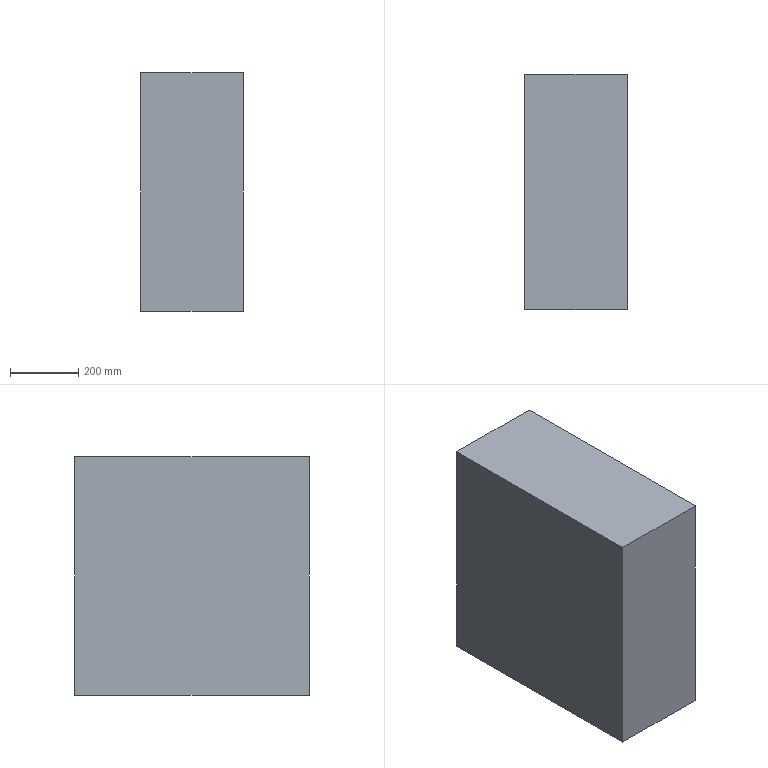Part | SolidWorks | features ICE 2, Extrusion 1 | 1 solid | 16 faces | box 300 x 690 x 700 mm | volume 37296000 mm3 | plane 16
STEP:
#1=CARTESIAN_POINT('',(-150.,345.,0.));
#2=VERTEX_POINT('',#1);
#3=CARTESIAN_POINT('',(-150.,-345.,0.));
#4=VERTEX_POINT('',#3);
#5=CARTESIAN_POINT('',(-150.,-345.,0.));
#6=DIRECTION('',(0.,-1.,0.));
#7=VECTOR('',#6,1000.);
#8=LINE('',#5,#7);
#9=EDGE_CURVE('',#2,#4,#8,.T.);
#10=ORIENTED_EDGE('',*,*,#9,.T.);
#11=CARTESIAN_POINT('',(-150.,-345.,700.));
#12=VERTEX_POINT('',#11);
#13=CARTESIAN_POINT('',(-150.,-345.,700.));
#14=DIRECTION('',(0.,0.,-1.));
#15=VECTOR('',#14,1000.);
#16=LINE('',#13,#15);
#17=EDGE_CURVE('',#12,#4,#16,.T.);
#18=ORIENTED_EDGE('',*,*,#17,.F.);
#19=CARTESIAN_POINT('',(-150.,345.,700.));
#20=VERTEX_POINT('',#19);
#21=CARTESIAN_POINT('',(-150.,-345.,700.));
#22=DIRECTION('',(0.,-1.,0.));
#23=VECTOR('',#22,1000.);
#24=LINE('',#21,#23);
#25=EDGE_CURVE('',#20,#12,#24,.T.);
#26=ORIENTED_EDGE('',*,*,#25,.F.);
#27=CARTESIAN_POINT('',(-150.,345.,700.));
#28=DIRECTION('',(0.,0.,-1.));
#29=VECTOR('',#28,1000.);
#30=LINE('',#27,#29);
#31=EDGE_CURVE('',#20,#2,#30,.T.);
#32=ORIENTED_EDGE('',*,*,#31,.T.);
#33=EDGE_LOOP('',(#10,#18,#26,#32));
#34=FACE_OUTER_BOUND('',#33,.T.);
#35=CARTESIAN_POINT('',(-150.,-345.,700.));
#36=DIRECTION('',(1.,0.,0.));
#37=DIRECTION('',(0.,0.,-1.));
#38=AXIS2_PLACEMENT_3D('',#35,#36,#37);
#39=PLANE('',#38);
#40=ADVANCED_FACE('',(#34),#39,.F.);
#41=CARTESIAN_POINT('',(150.,-345.,0.));
#42=VERTEX_POINT('',#41);
#43=CARTESIAN_POINT('',(150.,-345.,0.));
#44=DIRECTION('',(1.,0.,0.));
#45=VECTOR('',#44,1000.);
#46=LINE('',#43,#45);
#47=EDGE_CURVE('',#4,#42,#46,.T.);
#48=ORIENTED_EDGE('',*,*,#47,.T.);
#49=CARTESIAN_POINT('',(150.,-345.,700.));
#50=VERTEX_POINT('',#49);
#51=CARTESIAN_POINT('',(150.,-345.,700.));
#52=DIRECTION('',(0.,0.,-1.));
#53=VECTOR('',#52,1000.);
#54=LINE('',#51,#53);
#55=EDGE_CURVE('',#50,#42,#54,.T.);
#56=ORIENTED_EDGE('',*,*,#55,.F.);
#57=CARTESIAN_POINT('',(150.,-345.,700.));
#58=DIRECTION('',(1.,0.,0.));
#59=VECTOR('',#58,1000.);
#60=LINE('',#57,#59);
#61=EDGE_CURVE('',#12,#50,#60,.T.);
#62=ORIENTED_EDGE('',*,*,#61,.F.);
#63=ORIENTED_EDGE('',*,*,#17,.T.);
#64=EDGE_LOOP('',(#48,#56,#62,#63));
#65=FACE_OUTER_BOUND('',#64,.T.);
#66=CARTESIAN_POINT('',(150.,-345.,700.));
#67=DIRECTION('',(0.,1.,0.));
#68=DIRECTION('',(0.,0.,1.));
#69=AXIS2_PLACEMENT_3D('',#66,#67,#68);
#70=PLANE('',#69);
#71=ADVANCED_FACE('',(#65),#70,.F.);
#72=CARTESIAN_POINT('',(150.,-325.,665.));
#73=VERTEX_POINT('',#72);
#74=CARTESIAN_POINT('',(150.,-325.,35.));
#75=VERTEX_POINT('',#74);
#76=CARTESIAN_POINT('',(150.,-325.,35.));
#77=DIRECTION('',(0.,0.,-1.));
#78=VECTOR('',#77,1000.);
#79=LINE('',#76,#78);
#80=EDGE_CURVE('',#73,#75,#79,.T.);
#81=ORIENTED_EDGE('',*,*,#80,.F.);
#82=CARTESIAN_POINT('',(150.,135.,665.));
#83=VERTEX_POINT('',#82);
#84=CARTESIAN_POINT('',(150.,-325.,665.));
#85=DIRECTION('',(0.,-1.,0.));
#86=VECTOR('',#85,1000.);
#87=LINE('',#84,#86);
#88=EDGE_CURVE('',#83,#73,#87,.T.);
#89=ORIENTED_EDGE('',*,*,#88,.F.);
#90=CARTESIAN_POINT('',(150.,135.,35.));
#91=VERTEX_POINT('',#90);
#92=CARTESIAN_POINT('',(150.,135.,35.));
#93=DIRECTION('',(0.,0.,1.));
#94=VECTOR('',#93,1000.);
#95=LINE('',#92,#94);
#96=EDGE_CURVE('',#91,#83,#95,.T.);
#97=ORIENTED_EDGE('',*,*,#96,.F.);
#98=CARTESIAN_POINT('',(150.,-325.,35.));
#99=DIRECTION('',(0.,1.,0.));
#100=VECTOR('',#99,1000.);
#101=LINE('',#98,#100);
#102=EDGE_CURVE('',#75,#91,#101,.T.);
#103=ORIENTED_EDGE('',*,*,#102,.F.);
#104=EDGE_LOOP('',(#81,#89,#97,#103));
#105=FACE_BOUND('',#104,.T.);
#106=CARTESIAN_POINT('',(150.,175.,665.));
#107=VERTEX_POINT('',#106);
#108=CARTESIAN_POINT('',(150.,175.,35.));
#109=VERTEX_POINT('',#108);
#110=CARTESIAN_POINT('',(150.,175.,35.));
#111=DIRECTION('',(0.,0.,-1.));
#112=VECTOR('',#111,1000.);
#113=LINE('',#110,#112);
#114=EDGE_CURVE('',#107,#109,#113,.T.);
#115=ORIENTED_EDGE('',*,*,#114,.F.);
#116=CARTESIAN_POINT('',(150.,325.,665.));
#117=VERTEX_POINT('',#116);
#118=CARTESIAN_POINT('',(150.,175.,665.));
#119=DIRECTION('',(0.,-1.,0.));
#120=VECTOR('',#119,1000.);
#121=LINE('',#118,#120);
#122=EDGE_CURVE('',#117,#107,#121,.T.);
#123=ORIENTED_EDGE('',*,*,#122,.F.);
#124=CARTESIAN_POINT('',(150.,325.,35.));
#125=VERTEX_POINT('',#124);
#126=CARTESIAN_POINT('',(150.,325.,35.));
#127=DIRECTION('',(0.,0.,1.));
#128=VECTOR('',#127,1000.);
#129=LINE('',#126,#128);
#130=EDGE_CURVE('',#125,#117,#129,.T.);
#131=ORIENTED_EDGE('',*,*,#130,.F.);
#132=CARTESIAN_POINT('',(150.,175.,35.));
#133=DIRECTION('',(0.,1.,0.));
#134=VECTOR('',#133,1000.);
#135=LINE('',#132,#134);
#136=EDGE_CURVE('',#109,#125,#135,.T.);
#137=ORIENTED_EDGE('',*,*,#136,.F.);
#138=EDGE_LOOP('',(#115,#123,#131,#137));
#139=FACE_BOUND('',#138,.T.);
#140=CARTESIAN_POINT('',(150.,345.,0.));
#141=VERTEX_POINT('',#140);
#142=CARTESIAN_POINT('',(150.,-345.,0.));
#143=DIRECTION('',(0.,1.,0.));
#144=VECTOR('',#143,1000.);
#145=LINE('',#142,#144);
#146=EDGE_CURVE('',#42,#141,#145,.T.);
#147=ORIENTED_EDGE('',*,*,#146,.T.);
#148=CARTESIAN_POINT('',(150.,345.,700.));
#149=VERTEX_POINT('',#148);
#150=CARTESIAN_POINT('',(150.,345.,700.));
#151=DIRECTION('',(0.,0.,-1.));
#152=VECTOR('',#151,1000.);
#153=LINE('',#150,#152);
#154=EDGE_CURVE('',#149,#141,#153,.T.);
#155=ORIENTED_EDGE('',*,*,#154,.F.);
#156=CARTESIAN_POINT('',(150.,-345.,700.));
#157=DIRECTION('',(0.,1.,0.));
#158=VECTOR('',#157,1000.);
#159=LINE('',#156,#158);
#160=EDGE_CURVE('',#50,#149,#159,.T.);
#161=ORIENTED_EDGE('',*,*,#160,.F.);
#162=ORIENTED_EDGE('',*,*,#55,.T.);
#163=EDGE_LOOP('',(#147,#155,#161,#162));
#164=FACE_OUTER_BOUND('',#163,.T.);
#165=CARTESIAN_POINT('',(150.,-345.,700.));
#166=DIRECTION('',(-1.,0.,0.));
#167=DIRECTION('',(0.,0.,1.));
#168=AXIS2_PLACEMENT_3D('',#165,#166,#167);
#169=PLANE('',#168);
#170=ADVANCED_FACE('',(#105,#139,#164),#169,.F.);
#171=CARTESIAN_POINT('',(150.,345.,0.));
#172=DIRECTION('',(-1.,0.,0.));
#173=VECTOR('',#172,1000.);
#174=LINE('',#171,#173);
#175=EDGE_CURVE('',#141,#2,#174,.T.);
#176=ORIENTED_EDGE('',*,*,#175,.T.);
#177=ORIENTED_EDGE('',*,*,#31,.F.);
#178=CARTESIAN_POINT('',(150.,345.,700.));
#179=DIRECTION('',(-1.,0.,0.));
#180=VECTOR('',#179,1000.);
#181=LINE('',#178,#180);
#182=EDGE_CURVE('',#149,#20,#181,.T.);
#183=ORIENTED_EDGE('',*,*,#182,.F.);
#184=ORIENTED_EDGE('',*,*,#154,.T.);
#185=EDGE_LOOP('',(#176,#177,#183,#184));
#186=FACE_OUTER_BOUND('',#185,.T.);
#187=CARTESIAN_POINT('',(150.,345.,700.));
#188=DIRECTION('',(0.,-1.,0.));
#189=DIRECTION('',(0.,0.,-1.));
#190=AXIS2_PLACEMENT_3D('',#187,#188,#189);
#191=PLANE('',#190);
#192=ADVANCED_FACE('',(#186),#191,.F.);
#193=ORIENTED_EDGE('',*,*,#25,.T.);
#194=ORIENTED_EDGE('',*,*,#61,.T.);
#195=ORIENTED_EDGE('',*,*,#160,.T.);
#196=ORIENTED_EDGE('',*,*,#182,.T.);
#197=EDGE_LOOP('',(#193,#194,#195,#196));
#198=FACE_OUTER_BOUND('',#197,.T.);
#199=CARTESIAN_POINT('',(0.,0.,700.));
#200=DIRECTION('',(0.,0.,1.));
#201=DIRECTION('',(1.,0.,0.));
#202=AXIS2_PLACEMENT_3D('',#199,#200,#201);
#203=PLANE('',#202);
#204=ADVANCED_FACE('',(#198),#203,.T.);
#205=ORIENTED_EDGE('',*,*,#9,.F.);
#206=ORIENTED_EDGE('',*,*,#175,.F.);
#207=ORIENTED_EDGE('',*,*,#146,.F.);
#208=ORIENTED_EDGE('',*,*,#47,.F.);
#209=EDGE_LOOP('',(#205,#206,#207,#208));
#210=FACE_OUTER_BOUND('',#209,.T.);
#211=CARTESIAN_POINT('',(0.,0.,0.));
#212=DIRECTION('',(0.,0.,1.));
#213=DIRECTION('',(1.,0.,0.));
#214=AXIS2_PLACEMENT_3D('',#211,#212,#213);
#215=PLANE('',#214);
#216=ADVANCED_FACE('',(#210),#215,.F.);
#217=ORIENTED_EDGE('',*,*,#122,.T.);
#218=CARTESIAN_POINT('',(-130.,175.,665.));
#219=VERTEX_POINT('',#218);
#220=CARTESIAN_POINT('',(-130.,175.,665.));
#221=DIRECTION('',(1.,0.,0.));
#222=VECTOR('',#221,1000.);
#223=LINE('',#220,#222);
#224=EDGE_CURVE('',#219,#107,#223,.T.);
#225=ORIENTED_EDGE('',*,*,#224,.F.);
#226=CARTESIAN_POINT('',(-130.,325.,665.));
#227=VERTEX_POINT('',#226);
#228=CARTESIAN_POINT('',(-130.,175.,665.));
#229=DIRECTION('',(0.,-1.,0.));
#230=VECTOR('',#229,1000.);
#231=LINE('',#228,#230);
#232=EDGE_CURVE('',#227,#219,#231,.T.);
#233=ORIENTED_EDGE('',*,*,#232,.F.);
#234=CARTESIAN_POINT('',(-130.,325.,665.));
#235=DIRECTION('',(1.,0.,0.));
#236=VECTOR('',#235,1000.);
#237=LINE('',#234,#236);
#238=EDGE_CURVE('',#227,#117,#237,.T.);
#239=ORIENTED_EDGE('',*,*,#238,.T.);
#240=EDGE_LOOP('',(#217,#225,#233,#239));
#241=FACE_OUTER_BOUND('',#240,.T.);
#242=CARTESIAN_POINT('',(-130.,175.,665.));
#243=DIRECTION('',(0.,0.,1.));
#244=DIRECTION('',(1.,0.,0.));
#245=AXIS2_PLACEMENT_3D('',#242,#243,#244);
#246=PLANE('',#245);
#247=ADVANCED_FACE('',(#241),#246,.F.);
#248=ORIENTED_EDGE('',*,*,#130,.T.);
#249=ORIENTED_EDGE('',*,*,#238,.F.);
#250=CARTESIAN_POINT('',(-130.,325.,35.));
#251=VERTEX_POINT('',#250);
#252=CARTESIAN_POINT('',(-130.,325.,35.));
#253=DIRECTION('',(0.,0.,1.));
#254=VECTOR('',#253,1000.);
#255=LINE('',#252,#254);
#256=EDGE_CURVE('',#251,#227,#255,.T.);
#257=ORIENTED_EDGE('',*,*,#256,.F.);
#258=CARTESIAN_POINT('',(-130.,325.,35.));
#259=DIRECTION('',(1.,0.,0.));
#260=VECTOR('',#259,1000.);
#261=LINE('',#258,#260);
#262=EDGE_CURVE('',#251,#125,#261,.T.);
#263=ORIENTED_EDGE('',*,*,#262,.T.);
#264=EDGE_LOOP('',(#248,#249,#257,#263));
#265=FACE_OUTER_BOUND('',#264,.T.);
#266=CARTESIAN_POINT('',(-130.,325.,35.));
#267=DIRECTION('',(0.,1.,0.));
#268=DIRECTION('',(0.,0.,1.));
#269=AXIS2_PLACEMENT_3D('',#266,#267,#268);
#270=PLANE('',#269);
#271=ADVANCED_FACE('',(#265),#270,.F.);
#272=ORIENTED_EDGE('',*,*,#136,.T.);
#273=ORIENTED_EDGE('',*,*,#262,.F.);
#274=CARTESIAN_POINT('',(-130.,175.,35.));
#275=VERTEX_POINT('',#274);
#276=CARTESIAN_POINT('',(-130.,175.,35.));
#277=DIRECTION('',(0.,1.,0.));
#278=VECTOR('',#277,1000.);
#279=LINE('',#276,#278);
#280=EDGE_CURVE('',#275,#251,#279,.T.);
#281=ORIENTED_EDGE('',*,*,#280,.F.);
#282=CARTESIAN_POINT('',(-130.,175.,35.));
#283=DIRECTION('',(1.,0.,0.));
#284=VECTOR('',#283,1000.);
#285=LINE('',#282,#284);
#286=EDGE_CURVE('',#275,#109,#285,.T.);
#287=ORIENTED_EDGE('',*,*,#286,.T.);
#288=EDGE_LOOP('',(#272,#273,#281,#287));
#289=FACE_OUTER_BOUND('',#288,.T.);
#290=CARTESIAN_POINT('',(-130.,175.,35.));
#291=DIRECTION('',(0.,0.,-1.));
#292=DIRECTION('',(-1.,0.,0.));
#293=AXIS2_PLACEMENT_3D('',#290,#291,#292);
#294=PLANE('',#293);
#295=ADVANCED_FACE('',(#289),#294,.F.);
#296=ORIENTED_EDGE('',*,*,#114,.T.);
#297=ORIENTED_EDGE('',*,*,#286,.F.);
#298=CARTESIAN_POINT('',(-130.,175.,35.));
#299=DIRECTION('',(0.,0.,-1.));
#300=VECTOR('',#299,1000.);
#301=LINE('',#298,#300);
#302=EDGE_CURVE('',#219,#275,#301,.T.);
#303=ORIENTED_EDGE('',*,*,#302,.F.);
#304=ORIENTED_EDGE('',*,*,#224,.T.);
#305=EDGE_LOOP('',(#296,#297,#303,#304));
#306=FACE_OUTER_BOUND('',#305,.T.);
#307=CARTESIAN_POINT('',(-130.,175.,35.));
#308=DIRECTION('',(0.,-1.,0.));
#309=DIRECTION('',(0.,0.,-1.));
#310=AXIS2_PLACEMENT_3D('',#307,#308,#309);
#311=PLANE('',#310);
#312=ADVANCED_FACE('',(#306),#311,.F.);
#313=ORIENTED_EDGE('',*,*,#232,.T.);
#314=ORIENTED_EDGE('',*,*,#302,.T.);
#315=ORIENTED_EDGE('',*,*,#280,.T.);
#316=ORIENTED_EDGE('',*,*,#256,.T.);
#317=EDGE_LOOP('',(#313,#314,#315,#316));
#318=FACE_OUTER_BOUND('',#317,.T.);
#319=CARTESIAN_POINT('',(-130.,0.,0.));
#320=DIRECTION('',(1.,0.,0.));
#321=DIRECTION('',(0.,0.,-1.));
#322=AXIS2_PLACEMENT_3D('',#319,#320,#321);
#323=PLANE('',#322);
#324=ADVANCED_FACE('',(#318),#323,.T.);
#325=ORIENTED_EDGE('',*,*,#88,.T.);
#326=CARTESIAN_POINT('',(-130.,-325.,665.));
#327=VERTEX_POINT('',#326);
#328=CARTESIAN_POINT('',(-130.,-325.,665.));
#329=DIRECTION('',(1.,0.,0.));
#330=VECTOR('',#329,1000.);
#331=LINE('',#328,#330);
#332=EDGE_CURVE('',#327,#73,#331,.T.);
#333=ORIENTED_EDGE('',*,*,#332,.F.);
#334=CARTESIAN_POINT('',(-130.,135.,665.));
#335=VERTEX_POINT('',#334);
#336=CARTESIAN_POINT('',(-130.,-325.,665.));
#337=DIRECTION('',(0.,-1.,0.));
#338=VECTOR('',#337,1000.);
#339=LINE('',#336,#338);
#340=EDGE_CURVE('',#335,#327,#339,.T.);
#341=ORIENTED_EDGE('',*,*,#340,.F.);
#342=CARTESIAN_POINT('',(-130.,135.,665.));
#343=DIRECTION('',(1.,0.,0.));
#344=VECTOR('',#343,1000.);
#345=LINE('',#342,#344);
#346=EDGE_CURVE('',#335,#83,#345,.T.);
#347=ORIENTED_EDGE('',*,*,#346,.T.);
#348=EDGE_LOOP('',(#325,#333,#341,#347));
#349=FACE_OUTER_BOUND('',#348,.T.);
#350=CARTESIAN_POINT('',(-130.,-325.,665.));
#351=DIRECTION('',(0.,0.,1.));
#352=DIRECTION('',(1.,0.,0.));
#353=AXIS2_PLACEMENT_3D('',#350,#351,#352);
#354=PLANE('',#353);
#355=ADVANCED_FACE('',(#349),#354,.F.);
#356=ORIENTED_EDGE('',*,*,#96,.T.);
#357=ORIENTED_EDGE('',*,*,#346,.F.);
#358=CARTESIAN_POINT('',(-130.,135.,35.));
#359=VERTEX_POINT('',#358);
#360=CARTESIAN_POINT('',(-130.,135.,35.));
#361=DIRECTION('',(0.,0.,1.));
#362=VECTOR('',#361,1000.);
#363=LINE('',#360,#362);
#364=EDGE_CURVE('',#359,#335,#363,.T.);
#365=ORIENTED_EDGE('',*,*,#364,.F.);
#366=CARTESIAN_POINT('',(-130.,135.,35.));
#367=DIRECTION('',(1.,0.,0.));
#368=VECTOR('',#367,1000.);
#369=LINE('',#366,#368);
#370=EDGE_CURVE('',#359,#91,#369,.T.);
#371=ORIENTED_EDGE('',*,*,#370,.T.);
#372=EDGE_LOOP('',(#356,#357,#365,#371));
#373=FACE_OUTER_BOUND('',#372,.T.);
#374=CARTESIAN_POINT('',(-130.,135.,35.));
#375=DIRECTION('',(0.,1.,0.));
#376=DIRECTION('',(0.,0.,1.));
#377=AXIS2_PLACEMENT_3D('',#374,#375,#376);
#378=PLANE('',#377);
#379=ADVANCED_FACE('',(#373),#378,.F.);
#380=ORIENTED_EDGE('',*,*,#102,.T.);
#381=ORIENTED_EDGE('',*,*,#370,.F.);
#382=CARTESIAN_POINT('',(-130.,-325.,35.));
#383=VERTEX_POINT('',#382);
#384=CARTESIAN_POINT('',(-130.,-325.,35.));
#385=DIRECTION('',(0.,1.,0.));
#386=VECTOR('',#385,1000.);
#387=LINE('',#384,#386);
#388=EDGE_CURVE('',#383,#359,#387,.T.);
#389=ORIENTED_EDGE('',*,*,#388,.F.);
#390=CARTESIAN_POINT('',(-130.,-325.,35.));
#391=DIRECTION('',(1.,0.,0.));
#392=VECTOR('',#391,1000.);
#393=LINE('',#390,#392);
#394=EDGE_CURVE('',#383,#75,#393,.T.);
#395=ORIENTED_EDGE('',*,*,#394,.T.);
#396=EDGE_LOOP('',(#380,#381,#389,#395));
#397=FACE_OUTER_BOUND('',#396,.T.);
#398=CARTESIAN_POINT('',(-130.,-325.,35.));
#399=DIRECTION('',(0.,0.,-1.));
#400=DIRECTION('',(-1.,0.,0.));
#401=AXIS2_PLACEMENT_3D('',#398,#399,#400);
#402=PLANE('',#401);
#403=ADVANCED_FACE('',(#397),#402,.F.);
#404=ORIENTED_EDGE('',*,*,#80,.T.);
#405=ORIENTED_EDGE('',*,*,#394,.F.);
#406=CARTESIAN_POINT('',(-130.,-325.,35.));
#407=DIRECTION('',(0.,0.,-1.));
#408=VECTOR('',#407,1000.);
#409=LINE('',#406,#408);
#410=EDGE_CURVE('',#327,#383,#409,.T.);
#411=ORIENTED_EDGE('',*,*,#410,.F.);
#412=ORIENTED_EDGE('',*,*,#332,.T.);
#413=EDGE_LOOP('',(#404,#405,#411,#412));
#414=FACE_OUTER_BOUND('',#413,.T.);
#415=CARTESIAN_POINT('',(-130.,-325.,35.));
#416=DIRECTION('',(0.,-1.,0.));
#417=DIRECTION('',(0.,0.,-1.));
#418=AXIS2_PLACEMENT_3D('',#415,#416,#417);
#419=PLANE('',#418);
#420=ADVANCED_FACE('',(#414),#419,.F.);
#421=ORIENTED_EDGE('',*,*,#340,.T.);
#422=ORIENTED_EDGE('',*,*,#410,.T.);
#423=ORIENTED_EDGE('',*,*,#388,.T.);
#424=ORIENTED_EDGE('',*,*,#364,.T.);
#425=EDGE_LOOP('',(#421,#422,#423,#424));
#426=FACE_OUTER_BOUND('',#425,.T.);
#427=CARTESIAN_POINT('',(-130.,0.,0.));
#428=DIRECTION('',(1.,0.,0.));
#429=DIRECTION('',(0.,0.,-1.));
#430=AXIS2_PLACEMENT_3D('',#427,#428,#429);
#431=PLANE('',#430);
#432=ADVANCED_FACE('',(#426),#431,.T.);
#433=CLOSED_SHELL('',(#40,#71,#170,#192,#204,#216,#247,#271,#295,#312,#324,#355,#379,#403,#420,#432));
#434=MANIFOLD_SOLID_BREP('',#433);
#435=CARTESIAN_POINT('',(0.,0.,0.));
#436=DIRECTION('',(0.,0.,1.));
#437=DIRECTION('',(1.,0.,0.));
#438=AXIS2_PLACEMENT_3D('',#435,#436,#437);
#439=(LENGTH_UNIT()NAMED_UNIT(*)SI_UNIT(.MILLI.,.METRE.));
#440=UNCERTAINTY_MEASURE_WITH_UNIT(LENGTH_MEASURE(0.00001),#439,'','');
#441=(NAMED_UNIT(*)PLANE_ANGLE_UNIT()SI_UNIT($,.RADIAN.));
#442=(NAMED_UNIT(*)SI_UNIT($,.STERADIAN.)SOLID_ANGLE_UNIT());
#443=(GEOMETRIC_REPRESENTATION_CONTEXT(3)GLOBAL_UNCERTAINTY_ASSIGNED_CONTEXT((#440))GLOBAL_UNIT_ASSIGNED_CONTEXT((#439,#441,#442))REPRESENTATION_CONTEXT('',''));
#444=ADVANCED_BREP_SHAPE_REPRESENTATION('',(#434,#438),#443);